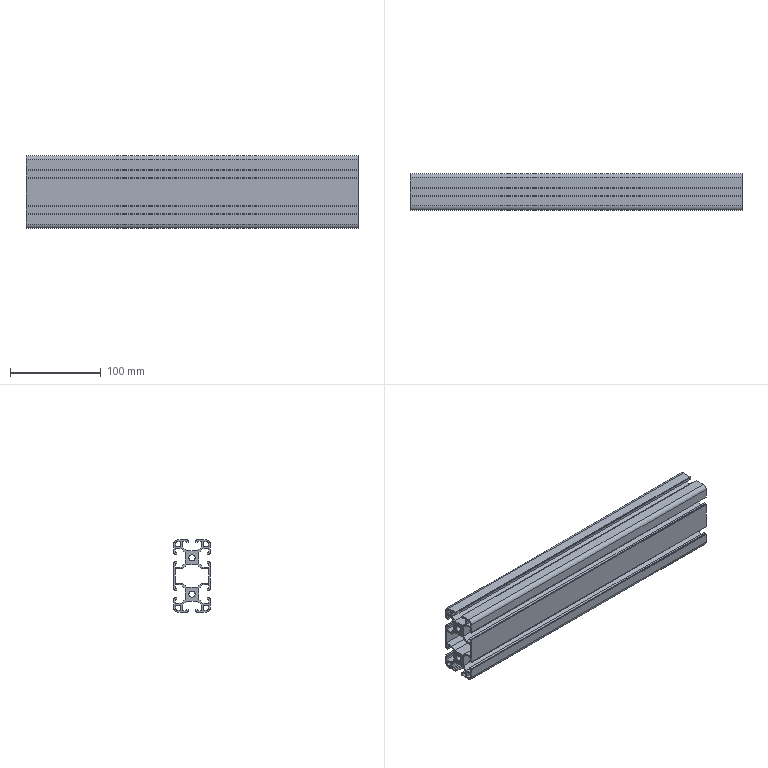Part | 1 solid | 155 faces | box 366 x 40.002 x 80 mm | volume 360288 mm3 | plane 142 | cylinder 13 | commonest cylinder face diameters 9 x5 5 x4 6.8 x4